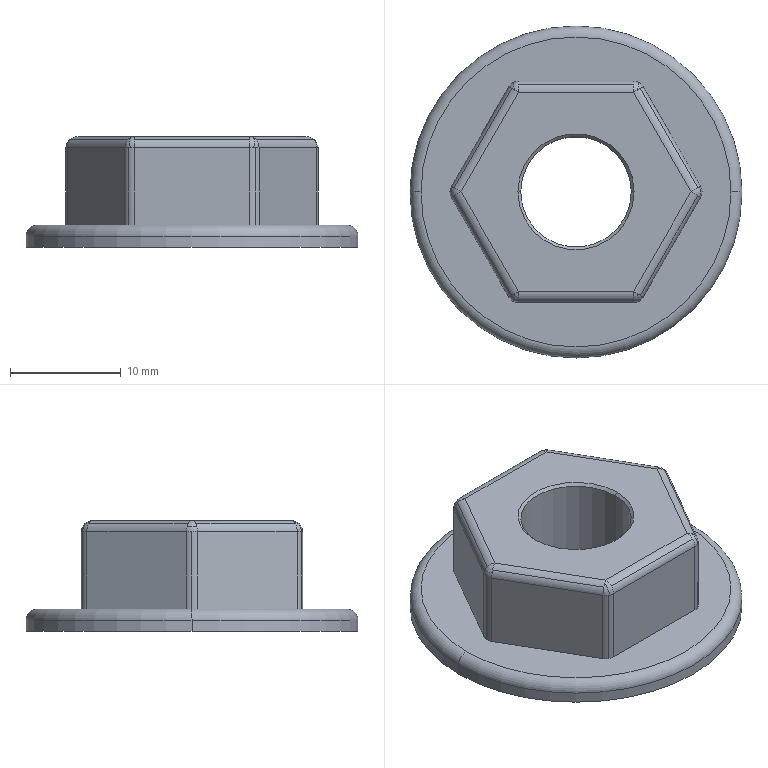Part | SolidWorks | features BaseBody 1 | 1 solid | 55 faces | box 30 x 30 x 10 mm | volume 3361 mm3 | cylinder 28 | sphere 12 | plane 9 | cone 4 | torus 2 | commonest cylinder face diameters 2 x24 10 x2 30 x2